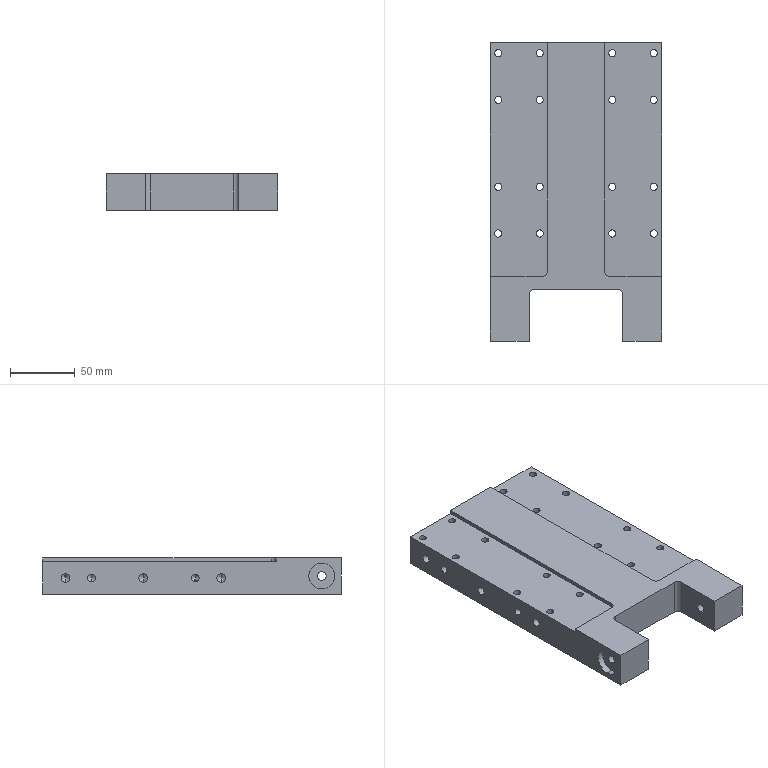Part | STEP file | LM-05-1260 | 1 solid | 150 faces | box 132 x 230 x 28 mm | volume 697857 mm3 | cylinder 96 | plane 34 | cone 20 | commonest cylinder face diameters 5.5 x32 9.5 x32 6.8 x16 6 x8 8 x4 20 x4